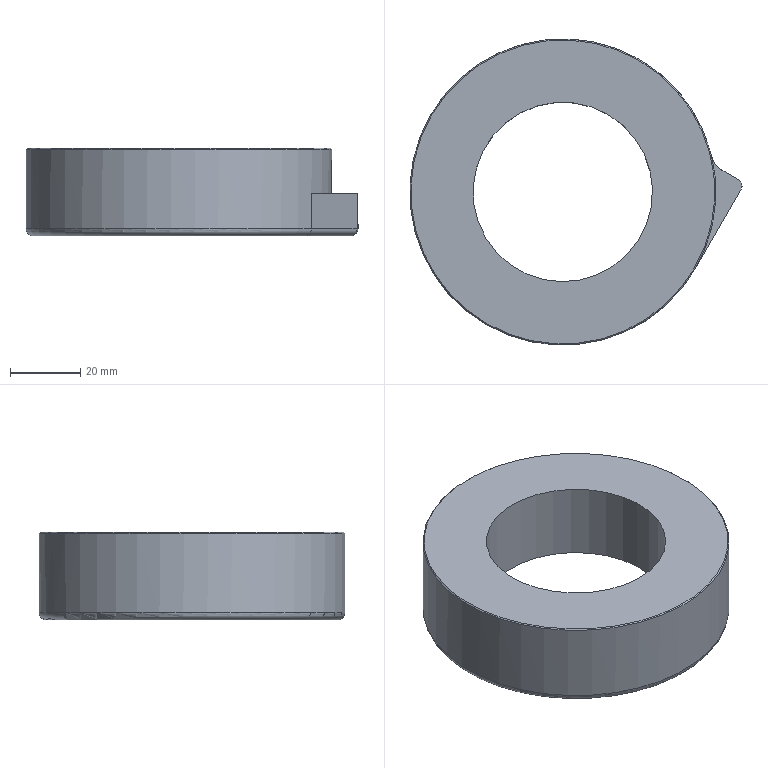Part | STEP file | 1 solid | 26 faces | box 94.44 x 87 x 25 mm | volume 90953 mm3 | plane 9 | cylinder 8 | cone 5 | torus 3 | sphere 1 | commonest cylinder face diameters 4 x3 14 x1 51 x1 71 x1 78.023 x1 87 x1
STEP:
#1=CARTESIAN_POINT('',(-37.672,21.75,-13.25));
#2=VERTEX_POINT('',#1);
#3=CARTESIAN_POINT('',(42.231,10.43,-13.25));
#4=VERTEX_POINT('',#3);
#5=CARTESIAN_POINT('',(0.,0.,-13.25));
#6=DIRECTION('',(0.,0.,-1.));
#7=DIRECTION('',(-0.866,0.5,0.));
#8=AXIS2_PLACEMENT_3D('',#5,#6,#7);
#9=CIRCLE('',#8,43.5);
#10=EDGE_CURVE('',#2,#4,#9,.T.);
#11=ORIENTED_EDGE('',*,*,#10,.T.);
#12=CARTESIAN_POINT('',(40.289,9.951,-15.25));
#13=VERTEX_POINT('',#12);
#14=CARTESIAN_POINT('',(40.289,9.951,-13.25));
#15=DIRECTION('',(-0.2398,0.9708,0.));
#16=DIRECTION('',(0.9708,0.2398,0.));
#17=AXIS2_PLACEMENT_3D('',#14,#15,#16);
#18=CIRCLE('',#17,2.);
#19=EDGE_CURVE('',#4,#13,#18,.T.);
#20=ORIENTED_EDGE('',*,*,#19,.T.);
#21=CARTESIAN_POINT('',(35.94,-20.75,-15.25));
#22=VERTEX_POINT('',#21);
#23=CARTESIAN_POINT('',(0.,0.,-15.25));
#24=DIRECTION('',(0.,0.,-1.));
#25=DIRECTION('',(0.866,-0.5,0.));
#26=AXIS2_PLACEMENT_3D('',#23,#24,#25);
#27=CIRCLE('',#26,41.5);
#28=EDGE_CURVE('',#22,#13,#27,.T.);
#29=ORIENTED_EDGE('',*,*,#28,.F.);
#30=CARTESIAN_POINT('',(37.672,-21.75,-13.25));
#31=VERTEX_POINT('',#30);
#32=CARTESIAN_POINT('',(35.94,-20.75,-13.25));
#33=DIRECTION('',(-0.5,-0.866,0.));
#34=DIRECTION('',(0.,0.,-1.));
#35=AXIS2_PLACEMENT_3D('',#32,#33,#34);
#36=CIRCLE('',#35,2.);
#37=EDGE_CURVE('',#22,#31,#36,.T.);
#38=ORIENTED_EDGE('',*,*,#37,.T.);
#39=CARTESIAN_POINT('',(37.672,-21.75,-13.25));
#40=CARTESIAN_POINT('',(37.217,-22.539,-13.25));
#41=CARTESIAN_POINT('',(36.256,-24.089,-13.25));
#42=CARTESIAN_POINT('',(34.671,-26.318,-13.25));
#43=CARTESIAN_POINT('',(32.95,-28.443,-13.25));
#44=CARTESIAN_POINT('',(31.099,-30.457,-13.25));
#45=CARTESIAN_POINT('',(29.125,-32.35,-13.25));
#46=CARTESIAN_POINT('',(27.036,-34.115,-13.25));
#47=CARTESIAN_POINT('',(24.84,-35.745,-13.25));
#48=CARTESIAN_POINT('',(22.546,-37.235,-13.25));
#49=CARTESIAN_POINT('',(20.163,-38.577,-13.25));
#50=CARTESIAN_POINT('',(17.701,-39.767,-13.25));
#51=CARTESIAN_POINT('',(15.168,-40.8,-13.25));
#52=CARTESIAN_POINT('',(12.576,-41.672,-13.25));
#53=CARTESIAN_POINT('',(9.934,-42.38,-13.25));
#54=CARTESIAN_POINT('',(7.253,-42.92,-13.25));
#55=CARTESIAN_POINT('',(4.543,-43.291,-13.25));
#56=CARTESIAN_POINT('',(1.816,-43.491,-13.25));
#57=CARTESIAN_POINT('',(-0.919,-43.519,-13.25));
#58=CARTESIAN_POINT('',(-3.65,-43.375,-13.25));
#59=CARTESIAN_POINT('',(-6.367,-43.06,-13.25));
#60=CARTESIAN_POINT('',(-9.059,-42.576,-13.25));
#61=CARTESIAN_POINT('',(-11.715,-41.923,-13.25));
#62=CARTESIAN_POINT('',(-14.324,-41.104,-13.25));
#63=CARTESIAN_POINT('',(-16.877,-40.124,-13.25));
#64=CARTESIAN_POINT('',(-19.364,-38.984,-13.25));
#65=CARTESIAN_POINT('',(-21.774,-37.691,-13.25));
#66=CARTESIAN_POINT('',(-24.098,-36.25,-13.25));
#67=CARTESIAN_POINT('',(-26.327,-34.665,-13.25));
#68=CARTESIAN_POINT('',(-28.452,-32.943,-13.25));
#69=CARTESIAN_POINT('',(-30.464,-31.091,-13.25));
#70=CARTESIAN_POINT('',(-32.357,-29.117,-13.25));
#71=CARTESIAN_POINT('',(-34.121,-27.027,-13.25));
#72=CARTESIAN_POINT('',(-35.751,-24.831,-13.25));
#73=CARTESIAN_POINT('',(-37.24,-22.537,-13.25));
#74=CARTESIAN_POINT('',(-38.582,-20.154,-13.25));
#75=CARTESIAN_POINT('',(-39.772,-17.691,-13.25));
#76=CARTESIAN_POINT('',(-40.804,-15.158,-13.25));
#77=CARTESIAN_POINT('',(-41.675,-12.566,-13.25));
#78=CARTESIAN_POINT('',(-42.382,-9.924,-13.25));
#79=CARTESIAN_POINT('',(-42.922,-7.242,-13.25));
#80=CARTESIAN_POINT('',(-43.292,-4.533,-13.25));
#81=CARTESIAN_POINT('',(-43.491,-1.805,-13.25));
#82=CARTESIAN_POINT('',(-43.519,0.9299,-13.25));
#83=CARTESIAN_POINT('',(-43.374,3.661,-13.25));
#84=CARTESIAN_POINT('',(-43.059,6.378,-13.25));
#85=CARTESIAN_POINT('',(-42.573,9.069,-13.25));
#86=CARTESIAN_POINT('',(-41.92,11.725,-13.25));
#87=CARTESIAN_POINT('',(-41.101,14.334,-13.25));
#88=CARTESIAN_POINT('',(-40.119,16.887,-13.25));
#89=CARTESIAN_POINT('',(-39.013,19.301,-13.25));
#90=CARTESIAN_POINT('',(-38.193,20.839,-13.25));
#91=CARTESIAN_POINT('',(-37.781,21.561,-13.25));
#92=CARTESIAN_POINT('',(-37.745,21.624,-13.25));
#93=CARTESIAN_POINT('',(-37.708,21.687,-13.25));
#94=CARTESIAN_POINT('',(-37.672,21.75,-13.25));
#95=B_SPLINE_CURVE_WITH_KNOTS('',3,(#39,#40,#41,#42,#43,#44,#45,#46,#47,#48,#49,#50,#51,#52,#53,#54,#55,#56,#57,#58,#59,#60,#61,#62,#63,#64,#65,#66,#67,#68,#69,#70,#71,#72,#73,#74,#75,#76,#77,#78,#79,#80,#81,#82,#83,#84,#85,#86,#87,#88,#89,#90,#91,#92,#93,#94),.UNSPECIFIED.,.F.,.F.,(4,1,1,1,1,1,1,1,1,1,1,1,1,1,1,1,1,1,1,1,1,1,1,1,1,1,1,1,1,1,1,1,1,1,1,1,1,1,1,1,1,1,1,1,1,1,1,1,1,1,3,4),(0.,0.02,0.04001,0.06001,0.08001,0.1,0.12,0.14,0.16,0.18,0.2,0.22,0.24,0.26,0.28,0.3,0.3201,0.3401,0.3601,0.3801,0.4001,0.4201,0.4401,0.4601,0.4801,0.5001,0.5201,0.5401,0.5601,0.5801,0.6001,0.6201,0.6401,0.6601,0.6801,0.7001,0.7201,0.7401,0.7601,0.7801,0.8001,0.8201,0.8401,0.8601,0.8801,0.9001,0.9201,0.9401,0.9602,0.9802,0.9984,1.),.UNSPECIFIED.);
#96=EDGE_CURVE('',#31,#2,#95,.T.);
#97=ORIENTED_EDGE('',*,*,#96,.T.);
#98=EDGE_LOOP('',(#11,#20,#29,#38,#97));
#99=FACE_BOUND('',#98,.T.);
#100=CARTESIAN_POINT('',(0.,0.,-13.25));
#101=DIRECTION('',(0.,0.,1.));
#102=DIRECTION('',(-0.8685,0.4956,0.));
#103=AXIS2_PLACEMENT_3D('',#100,#101,#102);
#104=TOROIDAL_SURFACE('',#103,41.5,2.);
#105=ADVANCED_FACE('',(#99),#104,.T.);
#106=ORIENTED_EDGE('',*,*,#28,.T.);
#107=CARTESIAN_POINT('',(44.527,4.315,-15.25));
#108=VERTEX_POINT('',#107);
#109=CARTESIAN_POINT('',(49.027,12.109,-15.25));
#110=DIRECTION('',(0.,0.,1.));
#111=DIRECTION('',(-0.9708,-0.2398,0.));
#112=AXIS2_PLACEMENT_3D('',#109,#110,#111);
#113=CIRCLE('',#112,9.);
#114=EDGE_CURVE('',#13,#108,#113,.T.);
#115=ORIENTED_EDGE('',*,*,#114,.T.);
#116=CARTESIAN_POINT('',(48.94,1.767,-15.25));
#117=VERTEX_POINT('',#116);
#118=CARTESIAN_POINT('',(48.94,1.767,-15.25));
#119=DIRECTION('',(-0.866,0.5,0.));
#120=VECTOR('',#119,1.);
#121=LINE('',#118,#120);
#122=EDGE_CURVE('',#117,#108,#121,.T.);
#123=ORIENTED_EDGE('',*,*,#122,.F.);
#124=CARTESIAN_POINT('',(35.94,-20.75,-15.25));
#125=DIRECTION('',(0.5,0.866,0.));
#126=VECTOR('',#125,1.);
#127=LINE('',#124,#126);
#128=EDGE_CURVE('',#22,#117,#127,.T.);
#129=ORIENTED_EDGE('',*,*,#128,.F.);
#130=EDGE_LOOP('',(#106,#115,#123,#129));
#131=FACE_BOUND('',#130,.T.);
#132=CARTESIAN_POINT('',(31.004,-17.9,-15.25));
#133=VERTEX_POINT('',#132);
#134=CARTESIAN_POINT('',(0.,0.,-15.25));
#135=DIRECTION('',(0.,0.,1.));
#136=DIRECTION('',(1.,0.,0.));
#137=AXIS2_PLACEMENT_3D('',#134,#135,#136);
#138=CIRCLE('',#137,35.8);
#139=EDGE_CURVE('',#133,#133,#138,.T.);
#140=ORIENTED_EDGE('',*,*,#139,.T.);
#141=EDGE_LOOP('',(#140));
#142=FACE_BOUND('',#141,.T.);
#143=CARTESIAN_POINT('',(-35.724,-20.625,-15.25));
#144=VERTEX_POINT('',#143);
#145=CARTESIAN_POINT('',(-34.425,-19.875,-15.25));
#146=VERTEX_POINT('',#145);
#147=CARTESIAN_POINT('',(-35.074,-20.25,-15.25));
#148=DIRECTION('',(0.,0.,1.));
#149=DIRECTION('',(-0.866,-0.5,0.));
#150=AXIS2_PLACEMENT_3D('',#147,#148,#149);
#151=CIRCLE('',#150,0.75);
#152=EDGE_CURVE('',#144,#146,#151,.T.);
#153=ORIENTED_EDGE('',*,*,#152,.T.);
#154=CARTESIAN_POINT('',(-35.074,-20.25,-15.25));
#155=DIRECTION('',(0.,0.,1.));
#156=DIRECTION('',(0.866,0.5,0.));
#157=AXIS2_PLACEMENT_3D('',#154,#155,#156);
#158=CIRCLE('',#157,0.75);
#159=EDGE_CURVE('',#146,#144,#158,.T.);
#160=ORIENTED_EDGE('',*,*,#159,.T.);
#161=EDGE_LOOP('',(#153,#160));
#162=FACE_BOUND('',#161,.T.);
#163=CARTESIAN_POINT('',(0.,0.,-15.25));
#164=DIRECTION('',(0.,0.,1.));
#165=DIRECTION('',(1.,0.,0.));
#166=AXIS2_PLACEMENT_3D('',#163,#164,#165);
#167=PLANE('',#166);
#168=ADVANCED_FACE('',(#131,#142,#162),#167,.F.);
#169=CARTESIAN_POINT('',(50.672,0.7667,-13.25));
#170=VERTEX_POINT('',#169);
#171=CARTESIAN_POINT('',(50.672,0.7667,-13.25));
#172=DIRECTION('',(-0.5,-0.866,0.));
#173=VECTOR('',#172,1.);
#174=LINE('',#171,#173);
#175=EDGE_CURVE('',#170,#31,#174,.T.);
#176=ORIENTED_EDGE('',*,*,#175,.T.);
#177=ORIENTED_EDGE('',*,*,#37,.F.);
#178=ORIENTED_EDGE('',*,*,#128,.T.);
#179=CARTESIAN_POINT('',(48.94,1.767,-13.25));
#180=DIRECTION('',(0.5,0.866,0.));
#181=DIRECTION('',(0.866,-0.5,0.));
#182=AXIS2_PLACEMENT_3D('',#179,#180,#181);
#183=CIRCLE('',#182,2.);
#184=EDGE_CURVE('',#170,#117,#183,.T.);
#185=ORIENTED_EDGE('',*,*,#184,.F.);
#186=EDGE_LOOP('',(#176,#177,#178,#185));
#187=FACE_BOUND('',#186,.T.);
#188=CARTESIAN_POINT('',(57.805,17.121,-13.25));
#189=DIRECTION('',(0.5,0.866,0.));
#190=DIRECTION('',(0.,0.,-1.));
#191=AXIS2_PLACEMENT_3D('',#188,#189,#190);
#192=CYLINDRICAL_SURFACE('',#191,2.);
#193=ADVANCED_FACE('',(#187),#192,.T.);
#194=ORIENTED_EDGE('',*,*,#184,.T.);
#195=CARTESIAN_POINT('',(49.94,3.499,-13.25));
#196=VERTEX_POINT('',#195);
#197=CARTESIAN_POINT('',(48.94,1.767,-13.25));
#198=DIRECTION('',(0.866,-0.5,0.));
#199=DIRECTION('',(0.,0.,-1.));
#200=AXIS2_PLACEMENT_3D('',#197,#198,#199);
#201=CIRCLE('',#200,2.);
#202=EDGE_CURVE('',#117,#196,#201,.T.);
#203=ORIENTED_EDGE('',*,*,#202,.T.);
#204=CARTESIAN_POINT('',(48.94,1.767,-13.25));
#205=DIRECTION('',(0.,0.,-1.));
#206=DIRECTION('',(0.5,0.866,0.));
#207=AXIS2_PLACEMENT_3D('',#204,#205,#206);
#208=CIRCLE('',#207,2.);
#209=EDGE_CURVE('',#196,#170,#208,.T.);
#210=ORIENTED_EDGE('',*,*,#209,.T.);
#211=EDGE_LOOP('',(#194,#203,#210));
#212=FACE_BOUND('',#211,.T.);
#213=CARTESIAN_POINT('',(48.94,1.767,-13.25));
#214=DIRECTION('',(0.5,0.866,0.));
#215=DIRECTION('',(0.,0.,1.));
#216=AXIS2_PLACEMENT_3D('',#213,#214,#215);
#217=SPHERICAL_SURFACE('',#216,2.);
#218=ADVANCED_FACE('',(#212),#217,.T.);
#219=CARTESIAN_POINT('',(50.491,3.03,-8.25));
#220=VERTEX_POINT('',#219);
#221=CARTESIAN_POINT('',(49.94,3.499,-10.321));
#222=VERTEX_POINT('',#221);
#223=CARTESIAN_POINT('',(50.491,3.03,-8.25));
#224=CARTESIAN_POINT('',(50.491,3.03,-8.283));
#225=CARTESIAN_POINT('',(50.49,3.03,-8.349));
#226=CARTESIAN_POINT('',(50.487,3.034,-8.447));
#227=CARTESIAN_POINT('',(50.483,3.039,-8.543));
#228=CARTESIAN_POINT('',(50.476,3.047,-8.639));
#229=CARTESIAN_POINT('',(50.468,3.057,-8.733));
#230=CARTESIAN_POINT('',(50.459,3.068,-8.825));
#231=CARTESIAN_POINT('',(50.448,3.081,-8.916));
#232=CARTESIAN_POINT('',(50.435,3.096,-9.005));
#233=CARTESIAN_POINT('',(50.42,3.112,-9.093));
#234=CARTESIAN_POINT('',(50.404,3.129,-9.179));
#235=CARTESIAN_POINT('',(50.387,3.148,-9.262));
#236=CARTESIAN_POINT('',(50.368,3.167,-9.343));
#237=CARTESIAN_POINT('',(50.348,3.187,-9.421));
#238=CARTESIAN_POINT('',(50.328,3.207,-9.496));
#239=CARTESIAN_POINT('',(50.306,3.228,-9.567));
#240=CARTESIAN_POINT('',(50.284,3.248,-9.636));
#241=CARTESIAN_POINT('',(50.261,3.269,-9.701));
#242=CARTESIAN_POINT('',(50.237,3.289,-9.763));
#243=CARTESIAN_POINT('',(50.214,3.308,-9.821));
#244=CARTESIAN_POINT('',(50.191,3.327,-9.876));
#245=CARTESIAN_POINT('',(50.168,3.345,-9.926));
#246=CARTESIAN_POINT('',(50.146,3.362,-9.974));
#247=CARTESIAN_POINT('',(50.124,3.379,-10.018));
#248=CARTESIAN_POINT('',(50.102,3.394,-10.059));
#249=CARTESIAN_POINT('',(50.081,3.409,-10.098));
#250=CARTESIAN_POINT('',(50.06,3.424,-10.135));
#251=CARTESIAN_POINT('',(50.04,3.437,-10.17));
#252=CARTESIAN_POINT('',(50.02,3.45,-10.203));
#253=CARTESIAN_POINT('',(50.,3.463,-10.234));
#254=CARTESIAN_POINT('',(49.98,3.475,-10.264));
#255=CARTESIAN_POINT('',(49.96,3.487,-10.293));
#256=CARTESIAN_POINT('',(49.947,3.495,-10.312));
#257=CARTESIAN_POINT('',(49.94,3.499,-10.321));
#258=B_SPLINE_CURVE_WITH_KNOTS('',3,(#223,#224,#225,#226,#227,#228,#229,#230,#231,#232,#233,#234,#235,#236,#237,#238,#239,#240,#241,#242,#243,#244,#245,#246,#247,#248,#249,#250,#251,#252,#253,#254,#255,#256,#257),.UNSPECIFIED.,.F.,.F.,(4,1,1,1,1,1,1,1,1,1,1,1,1,1,1,1,1,1,1,1,1,1,1,1,1,1,1,1,1,1,1,1,4),(0.,0.04051,0.08112,0.1217,0.162,0.202,0.2417,0.2813,0.3207,0.36,0.399,0.4375,0.4751,0.5122,0.5481,0.5832,0.6171,0.6505,0.6824,0.713,0.7417,0.7696,0.7954,0.82,0.8429,0.8655,0.8868,0.9074,0.9269,0.946,0.9644,0.9824,1.),.UNSPECIFIED.);
#259=EDGE_CURVE('',#220,#222,#258,.T.);
#260=ORIENTED_EDGE('',*,*,#259,.F.);
#261=CARTESIAN_POINT('',(49.94,3.499,-6.179));
#262=VERTEX_POINT('',#261);
#263=CARTESIAN_POINT('',(49.94,3.499,-6.179));
#264=CARTESIAN_POINT('',(49.954,3.491,-6.198));
#265=CARTESIAN_POINT('',(49.98,3.475,-6.236));
#266=CARTESIAN_POINT('',(50.018,3.451,-6.295));
#267=CARTESIAN_POINT('',(50.054,3.428,-6.355));
#268=CARTESIAN_POINT('',(50.089,3.404,-6.416));
#269=CARTESIAN_POINT('',(50.122,3.38,-6.478));
#270=CARTESIAN_POINT('',(50.154,3.357,-6.542));
#271=CARTESIAN_POINT('',(50.184,3.333,-6.607));
#272=CARTESIAN_POINT('',(50.212,3.31,-6.674));
#273=CARTESIAN_POINT('',(50.24,3.287,-6.742));
#274=CARTESIAN_POINT('',(50.265,3.265,-6.812));
#275=CARTESIAN_POINT('',(50.29,3.243,-6.882));
#276=CARTESIAN_POINT('',(50.312,3.222,-6.953));
#277=CARTESIAN_POINT('',(50.333,3.202,-7.024));
#278=CARTESIAN_POINT('',(50.353,3.183,-7.096));
#279=CARTESIAN_POINT('',(50.371,3.164,-7.168));
#280=CARTESIAN_POINT('',(50.387,3.147,-7.239));
#281=CARTESIAN_POINT('',(50.402,3.132,-7.31));
#282=CARTESIAN_POINT('',(50.415,3.117,-7.381));
#283=CARTESIAN_POINT('',(50.427,3.104,-7.451));
#284=CARTESIAN_POINT('',(50.438,3.092,-7.519));
#285=CARTESIAN_POINT('',(50.448,3.081,-7.585));
#286=CARTESIAN_POINT('',(50.456,3.071,-7.651));
#287=CARTESIAN_POINT('',(50.463,3.063,-7.714));
#288=CARTESIAN_POINT('',(50.469,3.056,-7.777));
#289=CARTESIAN_POINT('',(50.475,3.049,-7.838));
#290=CARTESIAN_POINT('',(50.479,3.044,-7.899));
#291=CARTESIAN_POINT('',(50.483,3.039,-7.959));
#292=CARTESIAN_POINT('',(50.486,3.036,-8.018));
#293=CARTESIAN_POINT('',(50.488,3.033,-8.077));
#294=CARTESIAN_POINT('',(50.49,3.031,-8.135));
#295=CARTESIAN_POINT('',(50.491,3.03,-8.193));
#296=CARTESIAN_POINT('',(50.491,3.03,-8.231));
#297=CARTESIAN_POINT('',(50.491,3.03,-8.25));
#298=B_SPLINE_CURVE_WITH_KNOTS('',3,(#263,#264,#265,#266,#267,#268,#269,#270,#271,#272,#273,#274,#275,#276,#277,#278,#279,#280,#281,#282,#283,#284,#285,#286,#287,#288,#289,#290,#291,#292,#293,#294,#295,#296,#297),.UNSPECIFIED.,.F.,.F.,(4,1,1,1,1,1,1,1,1,1,1,1,1,1,1,1,1,1,1,1,1,1,1,1,1,1,1,1,1,1,1,1,4),(0.,0.03654,0.07276,0.1087,0.1445,0.1802,0.2158,0.2514,0.2871,0.3229,0.3585,0.3941,0.4292,0.4641,0.4984,0.5324,0.5656,0.5986,0.6306,0.6619,0.692,0.7216,0.7498,0.7774,0.8039,0.8301,0.8557,0.8808,0.9052,0.9295,0.9533,0.9768,1.),.UNSPECIFIED.);
#299=EDGE_CURVE('',#262,#220,#298,.T.);
#300=ORIENTED_EDGE('',*,*,#299,.F.);
#301=CARTESIAN_POINT('',(49.94,3.499,-3.25));
#302=VERTEX_POINT('',#301);
#303=CARTESIAN_POINT('',(49.94,3.499,-6.179));
#304=DIRECTION('',(0.,0.,1.));
#305=VECTOR('',#304,1.);
#306=LINE('',#303,#305);
#307=EDGE_CURVE('',#262,#302,#306,.T.);
#308=ORIENTED_EDGE('',*,*,#307,.T.);
#309=CARTESIAN_POINT('',(50.672,0.7667,-3.25));
#310=VERTEX_POINT('',#309);
#311=CARTESIAN_POINT('',(48.94,1.767,-3.25));
#312=DIRECTION('',(0.,0.,1.));
#313=DIRECTION('',(0.866,-0.5,0.));
#314=AXIS2_PLACEMENT_3D('',#311,#312,#313);
#315=CIRCLE('',#314,2.);
#316=EDGE_CURVE('',#310,#302,#315,.T.);
#317=ORIENTED_EDGE('',*,*,#316,.F.);
#318=CARTESIAN_POINT('',(50.672,0.7667,-3.25));
#319=DIRECTION('',(0.,0.,-1.));
#320=VECTOR('',#319,1.);
#321=LINE('',#318,#320);
#322=EDGE_CURVE('',#310,#170,#321,.T.);
#323=ORIENTED_EDGE('',*,*,#322,.T.);
#324=ORIENTED_EDGE('',*,*,#209,.F.);
#325=CARTESIAN_POINT('',(49.94,3.499,-13.25));
#326=DIRECTION('',(0.,0.,1.));
#327=VECTOR('',#326,1.);
#328=LINE('',#325,#327);
#329=EDGE_CURVE('',#196,#222,#328,.T.);
#330=ORIENTED_EDGE('',*,*,#329,.T.);
#331=EDGE_LOOP('',(#260,#300,#308,#317,#323,#324,#330));
#332=FACE_BOUND('',#331,.T.);
#333=CARTESIAN_POINT('',(48.94,1.767,-15.25));
#334=DIRECTION('',(0.,0.,1.));
#335=DIRECTION('',(0.5,0.866,0.));
#336=AXIS2_PLACEMENT_3D('',#333,#334,#335);
#337=CYLINDRICAL_SURFACE('',#336,2.);
#338=ADVANCED_FACE('',(#332),#337,.T.);
#339=CARTESIAN_POINT('',(45.527,6.047,-10.199));
#340=VERTEX_POINT('',#339);
#341=CARTESIAN_POINT('',(47.775,4.749,-8.25));
#342=DIRECTION('',(-0.5,-0.866,0.));
#343=DIRECTION('',(-0.6925,0.3998,-0.6005));
#344=AXIS2_PLACEMENT_3D('',#341,#342,#343);
#345=CIRCLE('',#344,3.246);
#346=EDGE_CURVE('',#340,#222,#345,.T.);
#347=ORIENTED_EDGE('',*,*,#346,.T.);
#348=ORIENTED_EDGE('',*,*,#329,.F.);
#349=CARTESIAN_POINT('',(45.527,6.047,-13.25));
#350=VERTEX_POINT('',#349);
#351=CARTESIAN_POINT('',(45.527,6.047,-13.25));
#352=DIRECTION('',(0.866,-0.5,0.));
#353=VECTOR('',#352,1.);
#354=LINE('',#351,#353);
#355=EDGE_CURVE('',#350,#196,#354,.T.);
#356=ORIENTED_EDGE('',*,*,#355,.F.);
#357=CARTESIAN_POINT('',(45.527,6.047,-10.199));
#358=DIRECTION('',(0.,0.,-1.));
#359=VECTOR('',#358,1.);
#360=LINE('',#357,#359);
#361=EDGE_CURVE('',#340,#350,#360,.T.);
#362=ORIENTED_EDGE('',*,*,#361,.F.);
#363=EDGE_LOOP('',(#347,#348,#356,#362));
#364=FACE_BOUND('',#363,.T.);
#365=CARTESIAN_POINT('',(49.94,3.499,-15.25));
#366=DIRECTION('',(-0.5,-0.866,0.));
#367=DIRECTION('',(-0.866,0.5,0.));
#368=AXIS2_PLACEMENT_3D('',#365,#366,#367);
#369=PLANE('',#368);
#370=ADVANCED_FACE('',(#364),#369,.F.);
#371=CARTESIAN_POINT('',(45.527,6.047,-3.25));
#372=VERTEX_POINT('',#371);
#373=CARTESIAN_POINT('',(42.231,10.43,-3.25));
#374=VERTEX_POINT('',#373);
#375=CARTESIAN_POINT('',(49.027,12.109,-3.25));
#376=DIRECTION('',(0.,0.,-1.));
#377=DIRECTION('',(-0.5,-0.866,0.));
#378=AXIS2_PLACEMENT_3D('',#375,#376,#377);
#379=CIRCLE('',#378,7.);
#380=EDGE_CURVE('',#372,#374,#379,.T.);
#381=ORIENTED_EDGE('',*,*,#380,.F.);
#382=CARTESIAN_POINT('',(45.527,6.047,-6.301));
#383=VERTEX_POINT('',#382);
#384=CARTESIAN_POINT('',(45.527,6.047,-3.25));
#385=DIRECTION('',(0.,0.,-1.));
#386=VECTOR('',#385,1.);
#387=LINE('',#384,#386);
#388=EDGE_CURVE('',#372,#383,#387,.T.);
#389=ORIENTED_EDGE('',*,*,#388,.T.);
#390=CARTESIAN_POINT('',(45.527,6.047,-6.301));
#391=CARTESIAN_POINT('',(45.51,6.056,-6.326));
#392=CARTESIAN_POINT('',(45.478,6.075,-6.376));
#393=CARTESIAN_POINT('',(45.433,6.102,-6.454));
#394=CARTESIAN_POINT('',(45.39,6.128,-6.531));
#395=CARTESIAN_POINT('',(45.349,6.153,-6.61));
#396=CARTESIAN_POINT('',(45.306,6.18,-6.698));
#397=CARTESIAN_POINT('',(45.262,6.207,-6.797));
#398=CARTESIAN_POINT('',(45.218,6.236,-6.905));
#399=CARTESIAN_POINT('',(45.181,6.26,-7.005));
#400=CARTESIAN_POINT('',(45.15,6.28,-7.096));
#401=CARTESIAN_POINT('',(45.125,6.297,-7.178));
#402=CARTESIAN_POINT('',(45.102,6.313,-7.259));
#403=CARTESIAN_POINT('',(45.08,6.328,-7.343));
#404=CARTESIAN_POINT('',(45.059,6.342,-7.432));
#405=CARTESIAN_POINT('',(45.037,6.357,-7.541));
#406=CARTESIAN_POINT('',(45.015,6.372,-7.668));
#407=CARTESIAN_POINT('',(44.996,6.386,-7.808));
#408=CARTESIAN_POINT('',(44.984,6.394,-7.934));
#409=CARTESIAN_POINT('',(44.977,6.399,-8.042));
#410=CARTESIAN_POINT('',(44.973,6.402,-8.129));
#411=CARTESIAN_POINT('',(44.972,6.403,-8.197));
#412=CARTESIAN_POINT('',(44.972,6.403,-8.249));
#413=CARTESIAN_POINT('',(44.972,6.403,-8.309));
#414=CARTESIAN_POINT('',(44.974,6.402,-8.391));
#415=CARTESIAN_POINT('',(44.979,6.398,-8.495));
#416=CARTESIAN_POINT('',(44.987,6.392,-8.598));
#417=CARTESIAN_POINT('',(44.999,6.384,-8.71));
#418=CARTESIAN_POINT('',(45.015,6.372,-8.832));
#419=CARTESIAN_POINT('',(45.037,6.357,-8.958));
#420=CARTESIAN_POINT('',(45.064,6.339,-9.088));
#421=CARTESIAN_POINT('',(45.099,6.315,-9.234));
#422=CARTESIAN_POINT('',(45.149,6.281,-9.406));
#423=CARTESIAN_POINT('',(45.209,6.241,-9.575));
#424=CARTESIAN_POINT('',(45.265,6.205,-9.712));
#425=CARTESIAN_POINT('',(45.305,6.18,-9.8));
#426=CARTESIAN_POINT('',(45.334,6.162,-9.859));
#427=CARTESIAN_POINT('',(45.357,6.148,-9.906));
#428=CARTESIAN_POINT('',(45.381,6.133,-9.952));
#429=CARTESIAN_POINT('',(45.408,6.117,-10.001));
#430=CARTESIAN_POINT('',(45.437,6.099,-10.053));
#431=CARTESIAN_POINT('',(45.469,6.08,-10.108));
#432=CARTESIAN_POINT('',(45.499,6.063,-10.156));
#433=CARTESIAN_POINT('',(45.518,6.052,-10.187));
#434=CARTESIAN_POINT('',(45.527,6.047,-10.199));
#435=B_SPLINE_CURVE_WITH_KNOTS('',3,(#390,#391,#392,#393,#394,#395,#396,#397,#398,#399,#400,#401,#402,#403,#404,#405,#406,#407,#408,#409,#410,#411,#412,#413,#414,#415,#416,#417,#418,#419,#420,#421,#422,#423,#424,#425,#426,#427,#428,#429,#430,#431,#432,#433,#434),.UNSPECIFIED.,.F.,.F.,(4,1,1,1,1,1,1,1,1,1,1,1,1,1,1,1,1,1,1,1,1,1,1,1,1,1,1,1,1,1,1,1,1,1,1,1,1,1,1,1,1,1,4),(0.,0.02258,0.04492,0.06707,0.08901,0.1109,0.1399,0.1686,0.1971,0.2181,0.239,0.2595,0.2798,0.3019,0.326,0.3603,0.3943,0.4281,0.451,0.4717,0.4903,0.5,0.5089,0.5336,0.5585,0.5833,0.6081,0.6391,0.6719,0.7003,0.7353,0.7805,0.831,0.8669,0.8892,0.9026,0.9158,0.9286,0.9411,0.9572,0.973,0.9886,1.),.UNSPECIFIED.);
#436=EDGE_CURVE('',#383,#340,#435,.T.);
#437=ORIENTED_EDGE('',*,*,#436,.T.);
#438=ORIENTED_EDGE('',*,*,#361,.T.);
#439=CARTESIAN_POINT('',(49.027,12.109,-13.25));
#440=DIRECTION('',(0.,0.,1.));
#441=DIRECTION('',(-0.9708,-0.2398,0.));
#442=AXIS2_PLACEMENT_3D('',#439,#440,#441);
#443=CIRCLE('',#442,7.);
#444=EDGE_CURVE('',#4,#350,#443,.T.);
#445=ORIENTED_EDGE('',*,*,#444,.F.);
#446=CARTESIAN_POINT('',(42.231,10.43,-3.25));
#447=DIRECTION('',(0.,0.,-1.));
#448=VECTOR('',#447,1.);
#449=LINE('',#446,#448);
#450=EDGE_CURVE('',#374,#4,#449,.T.);
#451=ORIENTED_EDGE('',*,*,#450,.F.);
#452=EDGE_LOOP('',(#381,#389,#437,#438,#445,#451));
#453=FACE_BOUND('',#452,.T.);
#454=CARTESIAN_POINT('',(49.027,12.109,-15.25));
#455=DIRECTION('',(0.,0.,1.));
#456=DIRECTION('',(0.5,0.866,0.));
#457=AXIS2_PLACEMENT_3D('',#454,#455,#456);
#458=CYLINDRICAL_SURFACE('',#457,7.);
#459=ADVANCED_FACE('',(#453),#458,.F.);
#460=ORIENTED_EDGE('',*,*,#450,.T.);
#461=ORIENTED_EDGE('',*,*,#10,.F.);
#462=ORIENTED_EDGE('',*,*,#96,.F.);
#463=CARTESIAN_POINT('',(37.672,-21.75,-3.25));
#464=VERTEX_POINT('',#463);
#465=CARTESIAN_POINT('',(37.672,-21.75,-13.25));
#466=DIRECTION('',(0.,0.,1.));
#467=VECTOR('',#466,1.);
#468=LINE('',#465,#467);
#469=EDGE_CURVE('',#31,#464,#468,.T.);
#470=ORIENTED_EDGE('',*,*,#469,.T.);
#471=CARTESIAN_POINT('',(0.,0.,-3.25));
#472=DIRECTION('',(0.,0.,-1.));
#473=DIRECTION('',(0.9708,0.2398,0.));
#474=AXIS2_PLACEMENT_3D('',#471,#472,#473);
#475=CIRCLE('',#474,43.5);
#476=EDGE_CURVE('',#374,#464,#475,.T.);
#477=ORIENTED_EDGE('',*,*,#476,.F.);
#478=EDGE_LOOP('',(#460,#461,#462,#470,#477));
#479=FACE_BOUND('',#478,.T.);
#480=CARTESIAN_POINT('',(-37.672,21.75,9.45));
#481=VERTEX_POINT('',#480);
#482=CARTESIAN_POINT('',(-37.672,21.75,9.45));
#483=CARTESIAN_POINT('',(-38.128,20.961,9.45));
#484=CARTESIAN_POINT('',(-38.989,19.354,9.45));
#485=CARTESIAN_POINT('',(-40.128,16.867,9.45));
#486=CARTESIAN_POINT('',(-41.108,14.314,9.45));
#487=CARTESIAN_POINT('',(-41.926,11.704,9.45));
#488=CARTESIAN_POINT('',(-42.578,9.048,9.45));
#489=CARTESIAN_POINT('',(-43.062,6.356,9.45));
#490=CARTESIAN_POINT('',(-43.376,3.639,9.45));
#491=CARTESIAN_POINT('',(-43.519,0.9081,9.45));
#492=CARTESIAN_POINT('',(-43.49,-1.827,9.45));
#493=CARTESIAN_POINT('',(-43.29,-4.554,9.45));
#494=CARTESIAN_POINT('',(-42.918,-7.264,9.45));
#495=CARTESIAN_POINT('',(-42.377,-9.945,9.45));
#496=CARTESIAN_POINT('',(-41.669,-12.587,9.45));
#497=CARTESIAN_POINT('',(-40.796,-15.179,9.45));
#498=CARTESIAN_POINT('',(-39.763,-17.711,9.45));
#499=CARTESIAN_POINT('',(-38.572,-20.173,9.45));
#500=CARTESIAN_POINT('',(-37.229,-22.555,9.45));
#501=CARTESIAN_POINT('',(-35.739,-24.849,9.45));
#502=CARTESIAN_POINT('',(-34.108,-27.044,9.45));
#503=CARTESIAN_POINT('',(-32.342,-29.133,9.45));
#504=CARTESIAN_POINT('',(-30.449,-31.106,9.45));
#505=CARTESIAN_POINT('',(-28.435,-32.957,9.45));
#506=CARTESIAN_POINT('',(-26.309,-34.678,9.45));
#507=CARTESIAN_POINT('',(-24.08,-36.262,9.45));
#508=CARTESIAN_POINT('',(-21.755,-37.702,9.45));
#509=CARTESIAN_POINT('',(-19.344,-38.994,9.45));
#510=CARTESIAN_POINT('',(-16.857,-40.132,9.45));
#511=CARTESIAN_POINT('',(-14.304,-41.111,9.45));
#512=CARTESIAN_POINT('',(-11.694,-41.929,9.45));
#513=CARTESIAN_POINT('',(-9.037,-42.58,9.45));
#514=CARTESIAN_POINT('',(-6.345,-43.064,9.45));
#515=CARTESIAN_POINT('',(-3.629,-43.377,9.45));
#516=CARTESIAN_POINT('',(-0.8972,-43.519,9.45));
#517=CARTESIAN_POINT('',(1.838,-43.49,9.45));
#518=CARTESIAN_POINT('',(4.565,-43.289,9.45));
#519=CARTESIAN_POINT('',(7.275,-42.916,9.45));
#520=CARTESIAN_POINT('',(9.955,-42.375,9.45));
#521=CARTESIAN_POINT('',(12.597,-41.666,9.45));
#522=CARTESIAN_POINT('',(15.189,-40.793,9.45));
#523=CARTESIAN_POINT('',(17.721,-39.758,9.45));
#524=CARTESIAN_POINT('',(20.182,-38.567,9.45));
#525=CARTESIAN_POINT('',(22.565,-37.223,9.45));
#526=CARTESIAN_POINT('',(24.858,-35.733,9.45));
#527=CARTESIAN_POINT('',(27.053,-34.101,9.45));
#528=CARTESIAN_POINT('',(29.141,-32.335,9.45));
#529=CARTESIAN_POINT('',(31.114,-30.441,9.45));
#530=CARTESIAN_POINT('',(32.964,-28.427,9.45));
#531=CARTESIAN_POINT('',(34.684,-26.301,9.45));
#532=CARTESIAN_POINT('',(36.264,-24.077,9.45));
#533=CARTESIAN_POINT('',(37.22,-22.533,9.45));
#534=CARTESIAN_POINT('',(37.672,-21.75,9.45));
#535=CARTESIAN_POINT('',(38.128,-20.961,9.45));
#536=CARTESIAN_POINT('',(38.989,-19.354,9.45));
#537=CARTESIAN_POINT('',(40.128,-16.867,9.45));
#538=CARTESIAN_POINT('',(41.108,-14.314,9.45));
#539=CARTESIAN_POINT('',(41.926,-11.704,9.45));
#540=CARTESIAN_POINT('',(42.578,-9.048,9.45));
#541=CARTESIAN_POINT('',(43.062,-6.356,9.45));
#542=CARTESIAN_POINT('',(43.376,-3.639,9.45));
#543=CARTESIAN_POINT('',(43.519,-0.9081,9.45));
#544=CARTESIAN_POINT('',(43.49,1.827,9.45));
#545=CARTESIAN_POINT('',(43.29,4.554,9.45));
#546=CARTESIAN_POINT('',(42.918,7.264,9.45));
#547=CARTESIAN_POINT('',(42.377,9.945,9.45));
#548=CARTESIAN_POINT('',(41.669,12.587,9.45));
#549=CARTESIAN_POINT('',(40.796,15.179,9.45));
#550=CARTESIAN_POINT('',(39.763,17.711,9.45));
#551=CARTESIAN_POINT('',(38.572,20.173,9.45));
#552=CARTESIAN_POINT('',(37.229,22.555,9.45));
#553=CARTESIAN_POINT('',(35.739,24.849,9.45));
#554=CARTESIAN_POINT('',(34.108,27.044,9.45));
#555=CARTESIAN_POINT('',(32.342,29.133,9.45));
#556=CARTESIAN_POINT('',(30.449,31.106,9.45));
#557=CARTESIAN_POINT('',(28.435,32.957,9.45));
#558=CARTESIAN_POINT('',(26.309,34.678,9.45));
#559=CARTESIAN_POINT('',(24.08,36.262,9.45));
#560=CARTESIAN_POINT('',(21.755,37.702,9.45));
#561=CARTESIAN_POINT('',(19.344,38.994,9.45));
#562=CARTESIAN_POINT('',(16.857,40.132,9.45));
#563=CARTESIAN_POINT('',(14.304,41.111,9.45));
#564=CARTESIAN_POINT('',(11.694,41.929,9.45));
#565=CARTESIAN_POINT('',(9.037,42.58,9.45));
#566=CARTESIAN_POINT('',(6.345,43.064,9.45));
#567=CARTESIAN_POINT('',(3.629,43.377,9.45));
#568=CARTESIAN_POINT('',(0.8972,43.519,9.45));
#569=CARTESIAN_POINT('',(-1.838,43.49,9.45));
#570=CARTESIAN_POINT('',(-4.565,43.289,9.45));
#571=CARTESIAN_POINT('',(-7.275,42.916,9.45));
#572=CARTESIAN_POINT('',(-9.955,42.375,9.45));
#573=CARTESIAN_POINT('',(-12.597,41.666,9.45));
#574=CARTESIAN_POINT('',(-15.189,40.793,9.45));
#575=CARTESIAN_POINT('',(-17.721,39.758,9.45));
#576=CARTESIAN_POINT('',(-20.182,38.567,9.45));
#577=CARTESIAN_POINT('',(-22.565,37.223,9.45));
#578=CARTESIAN_POINT('',(-24.858,35.733,9.45));
#579=CARTESIAN_POINT('',(-27.053,34.101,9.45));
#580=CARTESIAN_POINT('',(-29.141,32.335,9.45));
#581=CARTESIAN_POINT('',(-31.114,30.441,9.45));
#582=CARTESIAN_POINT('',(-32.964,28.427,9.45));
#583=CARTESIAN_POINT('',(-34.684,26.301,9.45));
#584=CARTESIAN_POINT('',(-36.264,24.077,9.45));
#585=CARTESIAN_POINT('',(-37.22,22.533,9.45));
#586=CARTESIAN_POINT('',(-37.672,21.75,9.45));
#587=B_SPLINE_CURVE_WITH_KNOTS('',3,(#482,#483,#484,#485,#486,#487,#488,#489,#490,#491,#492,#493,#494,#495,#496,#497,#498,#499,#500,#501,#502,#503,#504,#505,#506,#507,#508,#509,#510,#511,#512,#513,#514,#515,#516,#517,#518,#519,#520,#521,#522,#523,#524,#525,#526,#527,#528,#529,#530,#531,#532,#533,#534,#535,#536,#537,#538,#539,#540,#541,#542,#543,#544,#545,#546,#547,#548,#549,#550,#551,#552,#553,#554,#555,#556,#557,#558,#559,#560,#561,#562,#563,#564,#565,#566,#567,#568,#569,#570,#571,#572,#573,#574,#575,#576,#577,#578,#579,#580,#581,#582,#583,#584,#585,#586),.UNSPECIFIED.,.T.,.F.,(4,1,1,1,1,1,1,1,1,1,1,1,1,1,1,1,1,1,1,1,1,1,1,1,1,1,1,1,1,1,1,1,1,1,1,1,1,1,1,1,1,1,1,1,1,1,1,1,1,1,3,1,1,1,1,1,1,1,1,1,1,1,1,1,1,1,1,1,1,1,1,1,1,1,1,1,1,1,1,1,1,1,1,1,1,1,1,1,1,1,1,1,1,1,1,1,1,1,1,1,4),(0.,0.01,0.02,0.03,0.04001,0.05001,0.06001,0.07001,0.08001,0.09001,0.1,0.11,0.12,0.13,0.14,0.15,0.16,0.17,0.18,0.19,0.2,0.21,0.22,0.23,0.24,0.25,0.26,0.27,0.28,0.29,0.3,0.31,0.3201,0.3301,0.3401,0.3501,0.3601,0.3701,0.3801,0.3901,0.4001,0.4101,0.4201,0.4301,0.4401,0.4501,0.4601,0.4701,0.4801,0.4901,0.5,0.51,0.52,0.53,0.54,0.55,0.56,0.57,0.58,0.59,0.6,0.61,0.62,0.63,0.64,0.65,0.66,0.67,0.68,0.69,0.7,0.71,0.72,0.73,0.74,0.75,0.76,0.77,0.78,0.79,0.8,0.81,0.8201,0.8301,0.8401,0.8501,0.8601,0.8701,0.8801,0.8901,0.9001,0.9101,0.9201,0.9301,0.9401,0.9501,0.9601,0.9701,0.9801,0.9901,1.),.UNSPECIFIED.);
#588=EDGE_CURVE('',#481,#481,#587,.T.);
#589=ORIENTED_EDGE('',*,*,#588,.F.);
#590=EDGE_LOOP('',(#589));
#591=FACE_OUTER_BOUND('',#590,.T.);
#592=CARTESIAN_POINT('',(0.,0.,9.75));
#593=DIRECTION('',(0.,0.,-1.));
#594=DIRECTION('',(-0.866,0.5,0.));
#595=AXIS2_PLACEMENT_3D('',#592,#593,#594);
#596=CYLINDRICAL_SURFACE('',#595,43.5);
#597=ADVANCED_FACE('',(#479,#591),#596,.T.);
#598=CARTESIAN_POINT('',(50.672,0.7667,-3.25));
#599=DIRECTION('',(-0.5,-0.866,0.));
#600=VECTOR('',#599,1.);
#601=LINE('',#598,#600);
#602=EDGE_CURVE('',#310,#464,#601,.T.);
#603=ORIENTED_EDGE('',*,*,#602,.T.);
#604=ORIENTED_EDGE('',*,*,#469,.F.);
#605=ORIENTED_EDGE('',*,*,#175,.F.);
#606=ORIENTED_EDGE('',*,*,#322,.F.);
#607=EDGE_LOOP('',(#603,#604,#605,#606));
#608=FACE_BOUND('',#607,.T.);
#609=CARTESIAN_POINT('',(37.672,-21.75,-15.25));
#610=DIRECTION('',(-0.866,0.5,0.));
#611=DIRECTION('',(0.,0.,1.));
#612=AXIS2_PLACEMENT_3D('',#609,#610,#611);
#613=PLANE('',#612);
#614=ADVANCED_FACE('',(#608),#613,.F.);
#615=CARTESIAN_POINT('',(45.527,6.047,-3.25));
#616=DIRECTION('',(0.866,-0.5,0.));
#617=VECTOR('',#616,1.);
#618=LINE('',#615,#617);
#619=EDGE_CURVE('',#372,#302,#618,.T.);
#620=ORIENTED_EDGE('',*,*,#619,.F.);
#621=ORIENTED_EDGE('',*,*,#380,.T.);
#622=ORIENTED_EDGE('',*,*,#476,.T.);
#623=ORIENTED_EDGE('',*,*,#602,.F.);
#624=ORIENTED_EDGE('',*,*,#316,.T.);
#625=EDGE_LOOP('',(#620,#621,#622,#623,#624));
#626=FACE_BOUND('',#625,.T.);
#627=CARTESIAN_POINT('',(0.,0.,-3.25));
#628=DIRECTION('',(0.,0.,1.));
#629=DIRECTION('',(1.,0.,0.));
#630=AXIS2_PLACEMENT_3D('',#627,#628,#629);
#631=PLANE('',#630);
#632=ADVANCED_FACE('',(#626),#631,.T.);
#633=ORIENTED_EDGE('',*,*,#619,.T.);
#634=ORIENTED_EDGE('',*,*,#307,.F.);
#635=CARTESIAN_POINT('',(47.775,4.749,-8.25));
#636=DIRECTION('',(-0.5,-0.866,0.));
#637=DIRECTION('',(0.6669,-0.385,0.638));
#638=AXIS2_PLACEMENT_3D('',#635,#636,#637);
#639=CIRCLE('',#638,3.246);
#640=EDGE_CURVE('',#262,#383,#639,.T.);
#641=ORIENTED_EDGE('',*,*,#640,.T.);
#642=ORIENTED_EDGE('',*,*,#388,.F.);
#643=EDGE_LOOP('',(#633,#634,#641,#642));
#644=FACE_BOUND('',#643,.T.);
#645=CARTESIAN_POINT('',(49.94,3.499,-15.25));
#646=DIRECTION('',(-0.5,-0.866,0.));
#647=DIRECTION('',(-0.866,0.5,0.));
#648=AXIS2_PLACEMENT_3D('',#645,#646,#647);
#649=PLANE('',#648);
#650=ADVANCED_FACE('',(#644),#649,.F.);
#651=ORIENTED_EDGE('',*,*,#259,.T.);
#652=ORIENTED_EDGE('',*,*,#346,.F.);
#653=ORIENTED_EDGE('',*,*,#436,.F.);
#654=ORIENTED_EDGE('',*,*,#640,.F.);
#655=ORIENTED_EDGE('',*,*,#299,.T.);
#656=EDGE_LOOP('',(#651,#652,#653,#654,#655));
#657=FACE_BOUND('',#656,.T.);
#658=CARTESIAN_POINT('',(50.22,2.759,-8.25));
#659=VERTEX_POINT('',#658);
#660=CARTESIAN_POINT('',(47.525,4.316,-8.25));
#661=DIRECTION('',(0.5,0.866,0.));
#662=DIRECTION('',(-0.866,0.5,0.));
#663=AXIS2_PLACEMENT_3D('',#660,#661,#662);
#664=CIRCLE('',#663,3.112);
#665=EDGE_CURVE('',#659,#659,#664,.T.);
#666=ORIENTED_EDGE('',*,*,#665,.F.);
#667=EDGE_LOOP('',(#666));
#668=FACE_OUTER_BOUND('',#667,.T.);
#669=CARTESIAN_POINT('',(47.658,4.546,-8.25));
#670=DIRECTION('',(0.5,0.866,0.));
#671=DIRECTION('',(0.866,-0.5,0.));
#672=AXIS2_PLACEMENT_3D('',#669,#670,#671);
#673=CONICAL_SURFACE('',#672,3.184,0.2618);
#674=ADVANCED_FACE('',(#657,#668),#673,.F.);
#675=ORIENTED_EDGE('',*,*,#665,.T.);
#676=EDGE_LOOP('',(#675));
#677=FACE_BOUND('',#676,.T.);
#678=CARTESIAN_POINT('',(13.75,23.816,-15.25));
#679=DIRECTION('',(-0.5,-0.866,0.));
#680=DIRECTION('',(-0.866,0.5,0.));
#681=AXIS2_PLACEMENT_3D('',#678,#679,#680);
#682=PLANE('',#681);
#683=ADVANCED_FACE('',(#677),#682,.F.);
#684=ORIENTED_EDGE('',*,*,#444,.T.);
#685=CARTESIAN_POINT('',(44.527,4.315,-13.25));
#686=DIRECTION('',(-0.866,0.5,0.));
#687=DIRECTION('',(0.5,0.866,0.));
#688=AXIS2_PLACEMENT_3D('',#685,#686,#687);
#689=CIRCLE('',#688,2.);
#690=EDGE_CURVE('',#350,#108,#689,.T.);
#691=ORIENTED_EDGE('',*,*,#690,.T.);
#692=ORIENTED_EDGE('',*,*,#114,.F.);
#693=ORIENTED_EDGE('',*,*,#19,.F.);
#694=EDGE_LOOP('',(#684,#691,#692,#693));
#695=FACE_BOUND('',#694,.T.);
#696=CARTESIAN_POINT('',(49.027,12.109,-13.25));
#697=DIRECTION('',(0.,0.,-1.));
#698=DIRECTION('',(-0.9778,-0.2094,0.));
#699=AXIS2_PLACEMENT_3D('',#696,#697,#698);
#700=TOROIDAL_SURFACE('',#699,9.,2.);
#701=ADVANCED_FACE('',(#695),#700,.T.);
#702=ORIENTED_EDGE('',*,*,#122,.T.);
#703=ORIENTED_EDGE('',*,*,#690,.F.);
#704=ORIENTED_EDGE('',*,*,#355,.T.);
#705=ORIENTED_EDGE('',*,*,#202,.F.);
#706=EDGE_LOOP('',(#702,#703,#704,#705));
#707=FACE_BOUND('',#706,.T.);
#708=CARTESIAN_POINT('',(-24.921,44.41,-13.25));
#709=DIRECTION('',(-0.866,0.5,0.));
#710=DIRECTION('',(0.,0.,-1.));
#711=AXIS2_PLACEMENT_3D('',#708,#709,#710);
#712=CYLINDRICAL_SURFACE('',#711,2.);
#713=ADVANCED_FACE('',(#707),#712,.T.);
#714=CARTESIAN_POINT('',(-37.412,21.6,9.75));
#715=VERTEX_POINT('',#714);
#716=CARTESIAN_POINT('',(0.,0.,9.75));
#717=DIRECTION('',(0.,0.,1.));
#718=DIRECTION('',(1.,0.,0.));
#719=AXIS2_PLACEMENT_3D('',#716,#717,#718);
#720=CIRCLE('',#719,43.2);
#721=EDGE_CURVE('',#715,#715,#720,.T.);
#722=ORIENTED_EDGE('',*,*,#721,.F.);
#723=EDGE_LOOP('',(#722));
#724=FACE_OUTER_BOUND('',#723,.T.);
#725=ORIENTED_EDGE('',*,*,#588,.T.);
#726=EDGE_LOOP('',(#725));
#727=FACE_OUTER_BOUND('',#726,.T.);
#728=CARTESIAN_POINT('',(0.,0.,9.6));
#729=DIRECTION('',(0.,0.,-1.));
#730=DIRECTION('',(-0.866,0.5,0.));
#731=AXIS2_PLACEMENT_3D('',#728,#729,#730);
#732=CONICAL_SURFACE('',#731,43.35,0.7854);
#733=ADVANCED_FACE('',(#724,#727),#732,.T.);
#734=ORIENTED_EDGE('',*,*,#721,.T.);
#735=EDGE_LOOP('',(#734));
#736=FACE_BOUND('',#735,.T.);
#737=CARTESIAN_POINT('',(12.75,22.084,9.75));
#738=VERTEX_POINT('',#737);
#739=CARTESIAN_POINT('',(0.,0.,9.75));
#740=DIRECTION('',(0.,0.,-1.));
#741=DIRECTION('',(-0.5,-0.866,0.));
#742=AXIS2_PLACEMENT_3D('',#739,#740,#741);
#743=CIRCLE('',#742,25.5);
#744=EDGE_CURVE('',#738,#738,#743,.T.);
#745=ORIENTED_EDGE('',*,*,#744,.T.);
#746=EDGE_LOOP('',(#745));
#747=FACE_BOUND('',#746,.T.);
#748=CARTESIAN_POINT('',(0.,0.,9.75));
#749=DIRECTION('',(0.,0.,1.));
#750=DIRECTION('',(1.,0.,0.));
#751=AXIS2_PLACEMENT_3D('',#748,#749,#750);
#752=PLANE('',#751);
#753=ADVANCED_FACE('',(#736,#747),#752,.T.);
#754=ORIENTED_EDGE('',*,*,#744,.F.);
#755=EDGE_LOOP('',(#754));
#756=FACE_OUTER_BOUND('',#755,.T.);
#757=CARTESIAN_POINT('',(12.75,22.084,-12.25));
#758=VERTEX_POINT('',#757);
#759=CARTESIAN_POINT('',(0.,0.,-12.25));
#760=DIRECTION('',(0.,0.,1.));
#761=DIRECTION('',(0.5,0.866,0.));
#762=AXIS2_PLACEMENT_3D('',#759,#760,#761);
#763=CIRCLE('',#762,25.5);
#764=EDGE_CURVE('',#758,#758,#763,.T.);
#765=ORIENTED_EDGE('',*,*,#764,.F.);
#766=EDGE_LOOP('',(#765));
#767=FACE_OUTER_BOUND('',#766,.T.);
#768=CARTESIAN_POINT('',(0.,0.,9.75));
#769=DIRECTION('',(0.,0.,-1.));
#770=DIRECTION('',(0.5,0.866,0.));
#771=AXIS2_PLACEMENT_3D('',#768,#769,#770);
#772=CYLINDRICAL_SURFACE('',#771,25.5);
#773=ADVANCED_FACE('',(#756,#767),#772,.F.);
#774=CARTESIAN_POINT('',(-19.506,-33.785,-12.25));
#775=VERTEX_POINT('',#774);
#776=CARTESIAN_POINT('',(0.,0.,-12.25));
#777=DIRECTION('',(0.,0.,-1.));
#778=DIRECTION('',(0.5,0.866,0.));
#779=AXIS2_PLACEMENT_3D('',#776,#777,#778);
#780=CIRCLE('',#779,39.011);
#781=EDGE_CURVE('',#775,#775,#780,.T.);
#782=ORIENTED_EDGE('',*,*,#781,.T.);
#783=EDGE_LOOP('',(#782));
#784=FACE_BOUND('',#783,.T.);
#785=ORIENTED_EDGE('',*,*,#764,.T.);
#786=EDGE_LOOP('',(#785));
#787=FACE_BOUND('',#786,.T.);
#788=CARTESIAN_POINT('',(0.,0.,-12.25));
#789=DIRECTION('',(0.,0.,1.));
#790=DIRECTION('',(1.,0.,0.));
#791=AXIS2_PLACEMENT_3D('',#788,#789,#790);
#792=PLANE('',#791);
#793=ADVANCED_FACE('',(#784,#787),#792,.F.);
#794=ORIENTED_EDGE('',*,*,#781,.F.);
#795=EDGE_LOOP('',(#794));
#796=FACE_OUTER_BOUND('',#795,.T.);
#797=CARTESIAN_POINT('',(-19.506,-33.785,-14.25));
#798=VERTEX_POINT('',#797);
#799=CARTESIAN_POINT('',(0.,0.,-14.25));
#800=DIRECTION('',(0.,0.,1.));
#801=DIRECTION('',(-0.5,-0.866,0.));
#802=AXIS2_PLACEMENT_3D('',#799,#800,#801);
#803=CIRCLE('',#802,39.011);
#804=EDGE_CURVE('',#798,#798,#803,.T.);
#805=ORIENTED_EDGE('',*,*,#804,.F.);
#806=EDGE_LOOP('',(#805));
#807=FACE_OUTER_BOUND('',#806,.T.);
#808=CARTESIAN_POINT('',(0.,0.,-11.25));
#809=DIRECTION('',(0.,0.,1.));
#810=DIRECTION('',(-0.5,-0.866,0.));
#811=AXIS2_PLACEMENT_3D('',#808,#809,#810);
#812=CYLINDRICAL_SURFACE('',#811,39.011);
#813=ADVANCED_FACE('',(#796,#807),#812,.F.);
#814=ORIENTED_EDGE('',*,*,#804,.T.);
#815=EDGE_LOOP('',(#814));
#816=FACE_BOUND('',#815,.T.);
#817=CARTESIAN_POINT('',(-31.177,18.,-14.25));
#818=VERTEX_POINT('',#817);
#819=CARTESIAN_POINT('',(0.,0.,-14.25));
#820=DIRECTION('',(0.,0.,-1.));
#821=DIRECTION('',(0.866,-0.5,0.));
#822=AXIS2_PLACEMENT_3D('',#819,#820,#821);
#823=CIRCLE('',#822,36.);
#824=EDGE_CURVE('',#818,#818,#823,.T.);
#825=ORIENTED_EDGE('',*,*,#824,.T.);
#826=EDGE_LOOP('',(#825));
#827=FACE_BOUND('',#826,.T.);
#828=CARTESIAN_POINT('',(0.,0.,-14.25));
#829=DIRECTION('',(0.,0.,-1.));
#830=DIRECTION('',(0.,-1.,0.));
#831=AXIS2_PLACEMENT_3D('',#828,#829,#830);
#832=PLANE('',#831);
#833=ADVANCED_FACE('',(#816,#827),#832,.F.);
#834=CARTESIAN_POINT('',(30.744,-17.75,-14.75));
#835=VERTEX_POINT('',#834);
#836=CARTESIAN_POINT('',(-30.744,17.75,-14.75));
#837=VERTEX_POINT('',#836);
#838=CARTESIAN_POINT('',(0.,0.,-14.75));
#839=DIRECTION('',(0.,0.,-1.));
#840=DIRECTION('',(0.866,-0.5,0.));
#841=AXIS2_PLACEMENT_3D('',#838,#839,#840);
#842=CIRCLE('',#841,35.5);
#843=EDGE_CURVE('',#835,#837,#842,.T.);
#844=ORIENTED_EDGE('',*,*,#843,.T.);
#845=CARTESIAN_POINT('',(0.,0.,-14.75));
#846=DIRECTION('',(0.,0.,-1.));
#847=DIRECTION('',(-0.866,0.5,0.));
#848=AXIS2_PLACEMENT_3D('',#845,#846,#847);
#849=CIRCLE('',#848,35.5);
#850=EDGE_CURVE('',#837,#835,#849,.T.);
#851=ORIENTED_EDGE('',*,*,#850,.T.);
#852=EDGE_LOOP('',(#844,#851));
#853=FACE_BOUND('',#852,.T.);
#854=ORIENTED_EDGE('',*,*,#824,.F.);
#855=EDGE_LOOP('',(#854));
#856=FACE_OUTER_BOUND('',#855,.T.);
#857=CARTESIAN_POINT('',(0.,0.,-14.75));
#858=DIRECTION('',(0.,0.,-1.));
#859=DIRECTION('',(0.866,-0.5,0.));
#860=AXIS2_PLACEMENT_3D('',#857,#858,#859);
#861=TOROIDAL_SURFACE('',#860,36.,0.5);
#862=ADVANCED_FACE('',(#853,#856),#861,.T.);
#863=ORIENTED_EDGE('',*,*,#850,.F.);
#864=ORIENTED_EDGE('',*,*,#843,.F.);
#865=EDGE_LOOP('',(#863,#864));
#866=FACE_BOUND('',#865,.T.);
#867=CARTESIAN_POINT('',(30.744,-17.75,-14.95));
#868=VERTEX_POINT('',#867);
#869=CARTESIAN_POINT('',(30.744,-17.75,-14.95));
#870=CARTESIAN_POINT('',(31.116,-17.106,-14.95));
#871=CARTESIAN_POINT('',(31.819,-15.795,-14.95));
#872=CARTESIAN_POINT('',(32.748,-13.765,-14.95));
#873=CARTESIAN_POINT('',(33.548,-11.681,-14.95));
#874=CARTESIAN_POINT('',(34.215,-9.552,-14.95));
#875=CARTESIAN_POINT('',(34.747,-7.384,-14.95));
#876=CARTESIAN_POINT('',(35.143,-5.187,-14.95));
#877=CARTESIAN_POINT('',(35.399,-2.97,-14.95));
#878=CARTESIAN_POINT('',(35.516,-0.7411,-14.95));
#879=CARTESIAN_POINT('',(35.492,1.491,-14.95));
#880=CARTESIAN_POINT('',(35.328,3.717,-14.95));
#881=CARTESIAN_POINT('',(35.025,5.928,-14.95));
#882=CARTESIAN_POINT('',(34.584,8.116,-14.95));
#883=CARTESIAN_POINT('',(34.006,10.272,-14.95));
#884=CARTESIAN_POINT('',(33.294,12.387,-14.95));
#885=CARTESIAN_POINT('',(32.45,14.454,-14.95));
#886=CARTESIAN_POINT('',(31.478,16.463,-14.95));
#887=CARTESIAN_POINT('',(30.382,18.407,-14.95));
#888=CARTESIAN_POINT('',(29.166,20.279,-14.95));
#889=CARTESIAN_POINT('',(27.835,22.071,-14.95));
#890=CARTESIAN_POINT('',(26.394,23.775,-14.95));
#891=CARTESIAN_POINT('',(24.849,25.386,-14.95));
#892=CARTESIAN_POINT('',(23.206,26.896,-14.95));
#893=CARTESIAN_POINT('',(21.471,28.3,-14.95));
#894=CARTESIAN_POINT('',(19.651,29.593,-14.95));
#895=CARTESIAN_POINT('',(17.754,30.769,-14.95));
#896=CARTESIAN_POINT('',(15.787,31.823,-14.95));
#897=CARTESIAN_POINT('',(13.757,32.751,-14.95));
#898=CARTESIAN_POINT('',(11.673,33.551,-14.95));
#899=CARTESIAN_POINT('',(9.543,34.218,-14.95));
#900=CARTESIAN_POINT('',(7.375,34.749,-14.95));
#901=CARTESIAN_POINT('',(5.178,35.144,-14.95));
#902=CARTESIAN_POINT('',(2.961,35.4,-14.95));
#903=CARTESIAN_POINT('',(0.7322,35.516,-14.95));
#904=CARTESIAN_POINT('',(-1.5,35.492,-14.95));
#905=CARTESIAN_POINT('',(-3.726,35.327,-14.95));
#906=CARTESIAN_POINT('',(-5.937,35.024,-14.95));
#907=CARTESIAN_POINT('',(-8.125,34.582,-14.95));
#908=CARTESIAN_POINT('',(-10.28,34.003,-14.95));
#909=CARTESIAN_POINT('',(-12.395,33.291,-14.95));
#910=CARTESIAN_POINT('',(-14.462,32.446,-14.95));
#911=CARTESIAN_POINT('',(-16.471,31.474,-14.95));
#912=CARTESIAN_POINT('',(-18.415,30.378,-14.95));
#913=CARTESIAN_POINT('',(-20.286,29.161,-14.95));
#914=CARTESIAN_POINT('',(-22.078,27.83,-14.95));
#915=CARTESIAN_POINT('',(-23.782,26.388,-14.95));
#916=CARTESIAN_POINT('',(-25.392,24.843,-14.95));
#917=CARTESIAN_POINT('',(-26.902,23.199,-14.95));
#918=CARTESIAN_POINT('',(-28.306,21.464,-14.95));
#919=CARTESIAN_POINT('',(-29.594,19.649,-14.95));
#920=CARTESIAN_POINT('',(-30.375,18.389,-14.95));
#921=CARTESIAN_POINT('',(-30.744,17.75,-14.95));
#922=CARTESIAN_POINT('',(-31.116,17.106,-14.95));
#923=CARTESIAN_POINT('',(-31.819,15.795,-14.95));
#924=CARTESIAN_POINT('',(-32.748,13.765,-14.95));
#925=CARTESIAN_POINT('',(-33.548,11.681,-14.95));
#926=CARTESIAN_POINT('',(-34.215,9.552,-14.95));
#927=CARTESIAN_POINT('',(-34.747,7.384,-14.95));
#928=CARTESIAN_POINT('',(-35.143,5.187,-14.95));
#929=CARTESIAN_POINT('',(-35.399,2.97,-14.95));
#930=CARTESIAN_POINT('',(-35.516,0.7411,-14.95));
#931=CARTESIAN_POINT('',(-35.492,-1.491,-14.95));
#932=CARTESIAN_POINT('',(-35.328,-3.717,-14.95));
#933=CARTESIAN_POINT('',(-35.025,-5.928,-14.95));
#934=CARTESIAN_POINT('',(-34.584,-8.116,-14.95));
#935=CARTESIAN_POINT('',(-34.006,-10.272,-14.95));
#936=CARTESIAN_POINT('',(-33.294,-12.387,-14.95));
#937=CARTESIAN_POINT('',(-32.45,-14.454,-14.95));
#938=CARTESIAN_POINT('',(-31.478,-16.463,-14.95));
#939=CARTESIAN_POINT('',(-30.382,-18.407,-14.95));
#940=CARTESIAN_POINT('',(-29.166,-20.279,-14.95));
#941=CARTESIAN_POINT('',(-27.835,-22.071,-14.95));
#942=CARTESIAN_POINT('',(-26.394,-23.775,-14.95));
#943=CARTESIAN_POINT('',(-24.849,-25.386,-14.95));
#944=CARTESIAN_POINT('',(-23.206,-26.896,-14.95));
#945=CARTESIAN_POINT('',(-21.471,-28.3,-14.95));
#946=CARTESIAN_POINT('',(-19.651,-29.593,-14.95));
#947=CARTESIAN_POINT('',(-17.754,-30.769,-14.95));
#948=CARTESIAN_POINT('',(-15.787,-31.823,-14.95));
#949=CARTESIAN_POINT('',(-13.757,-32.751,-14.95));
#950=CARTESIAN_POINT('',(-11.673,-33.551,-14.95));
#951=CARTESIAN_POINT('',(-9.543,-34.218,-14.95));
#952=CARTESIAN_POINT('',(-7.375,-34.749,-14.95));
#953=CARTESIAN_POINT('',(-5.178,-35.144,-14.95));
#954=CARTESIAN_POINT('',(-2.961,-35.4,-14.95));
#955=CARTESIAN_POINT('',(-0.7322,-35.516,-14.95));
#956=CARTESIAN_POINT('',(1.5,-35.492,-14.95));
#957=CARTESIAN_POINT('',(3.726,-35.327,-14.95));
#958=CARTESIAN_POINT('',(5.937,-35.024,-14.95));
#959=CARTESIAN_POINT('',(8.125,-34.582,-14.95));
#960=CARTESIAN_POINT('',(10.28,-34.003,-14.95));
#961=CARTESIAN_POINT('',(12.395,-33.291,-14.95));
#962=CARTESIAN_POINT('',(14.462,-32.446,-14.95));
#963=CARTESIAN_POINT('',(16.471,-31.474,-14.95));
#964=CARTESIAN_POINT('',(18.415,-30.378,-14.95));
#965=CARTESIAN_POINT('',(20.286,-29.161,-14.95));
#966=CARTESIAN_POINT('',(22.078,-27.83,-14.95));
#967=CARTESIAN_POINT('',(23.782,-26.388,-14.95));
#968=CARTESIAN_POINT('',(25.392,-24.843,-14.95));
#969=CARTESIAN_POINT('',(26.902,-23.199,-14.95));
#970=CARTESIAN_POINT('',(28.306,-21.464,-14.95));
#971=CARTESIAN_POINT('',(29.594,-19.649,-14.95));
#972=CARTESIAN_POINT('',(30.375,-18.389,-14.95));
#973=CARTESIAN_POINT('',(30.744,-17.75,-14.95));
#974=B_SPLINE_CURVE_WITH_KNOTS('',3,(#869,#870,#871,#872,#873,#874,#875,#876,#877,#878,#879,#880,#881,#882,#883,#884,#885,#886,#887,#888,#889,#890,#891,#892,#893,#894,#895,#896,#897,#898,#899,#900,#901,#902,#903,#904,#905,#906,#907,#908,#909,#910,#911,#912,#913,#914,#915,#916,#917,#918,#919,#920,#921,#922,#923,#924,#925,#926,#927,#928,#929,#930,#931,#932,#933,#934,#935,#936,#937,#938,#939,#940,#941,#942,#943,#944,#945,#946,#947,#948,#949,#950,#951,#952,#953,#954,#955,#956,#957,#958,#959,#960,#961,#962,#963,#964,#965,#966,#967,#968,#969,#970,#971,#972,#973),.UNSPECIFIED.,.T.,.F.,(4,1,1,1,1,1,1,1,1,1,1,1,1,1,1,1,1,1,1,1,1,1,1,1,1,1,1,1,1,1,1,1,1,1,1,1,1,1,1,1,1,1,1,1,1,1,1,1,1,1,3,1,1,1,1,1,1,1,1,1,1,1,1,1,1,1,1,1,1,1,1,1,1,1,1,1,1,1,1,1,1,1,1,1,1,1,1,1,1,1,1,1,1,1,1,1,1,1,1,1,4),(0.,0.01,0.02,0.03,0.04001,0.05001,0.06001,0.07001,0.08001,0.09001,0.1,0.11,0.12,0.13,0.14,0.15,0.16,0.17,0.18,0.19,0.2,0.21,0.22,0.23,0.24,0.25,0.26,0.27,0.28,0.29,0.3,0.31,0.3201,0.3301,0.3401,0.3501,0.3601,0.3701,0.3801,0.3901,0.4001,0.4101,0.4201,0.4301,0.4401,0.4501,0.4601,0.4701,0.4801,0.4901,0.5,0.51,0.52,0.53,0.54,0.55,0.56,0.57,0.58,0.59,0.6,0.61,0.62,0.63,0.64,0.65,0.66,0.67,0.68,0.69,0.7,0.71,0.72,0.73,0.74,0.75,0.76,0.77,0.78,0.79,0.8,0.81,0.8201,0.8301,0.8401,0.8501,0.8601,0.8701,0.8801,0.8901,0.9001,0.9101,0.9201,0.9301,0.9401,0.9501,0.9601,0.9701,0.9801,0.9901,1.),.UNSPECIFIED.);
#975=EDGE_CURVE('',#868,#868,#974,.T.);
#976=ORIENTED_EDGE('',*,*,#975,.F.);
#977=EDGE_LOOP('',(#976));
#978=FACE_OUTER_BOUND('',#977,.T.);
#979=CARTESIAN_POINT('',(0.,0.,-14.2));
#980=DIRECTION('',(0.,0.,1.));
#981=DIRECTION('',(-0.866,0.5,0.));
#982=AXIS2_PLACEMENT_3D('',#979,#980,#981);
#983=CYLINDRICAL_SURFACE('',#982,35.5);
#984=ADVANCED_FACE('',(#866,#978),#983,.F.);
#985=ORIENTED_EDGE('',*,*,#139,.F.);
#986=EDGE_LOOP('',(#985));
#987=FACE_OUTER_BOUND('',#986,.T.);
#988=ORIENTED_EDGE('',*,*,#975,.T.);
#989=EDGE_LOOP('',(#988));
#990=FACE_OUTER_BOUND('',#989,.T.);
#991=CARTESIAN_POINT('',(0.,0.,-15.1));
#992=DIRECTION('',(0.,0.,-1.));
#993=DIRECTION('',(-0.866,0.5,0.));
#994=AXIS2_PLACEMENT_3D('',#991,#992,#993);
#995=CONICAL_SURFACE('',#994,35.65,0.7854);
#996=ADVANCED_FACE('',(#987,#990),#995,.F.);
#997=CARTESIAN_POINT('',(-35.074,-20.25,-14.5));
#998=VERTEX_POINT('',#997);
#999=CARTESIAN_POINT('',(-35.074,-20.25,-14.5));
#1000=DIRECTION('',(0.6124,0.3536,-0.7071));
#1001=VECTOR('',#1000,1.);
#1002=LINE('',#999,#1001);
#1003=EDGE_CURVE('',#998,#146,#1002,.T.);
#1004=ORIENTED_EDGE('',*,*,#1003,.F.);
#1005=CARTESIAN_POINT('',(-35.724,-20.625,-15.25));
#1006=DIRECTION('',(0.6124,0.3536,0.7071));
#1007=VECTOR('',#1006,1.);
#1008=LINE('',#1005,#1007);
#1009=EDGE_CURVE('',#144,#998,#1008,.T.);
#1010=ORIENTED_EDGE('',*,*,#1009,.F.);
#1011=ORIENTED_EDGE('',*,*,#159,.F.);
#1012=EDGE_LOOP('',(#1004,#1010,#1011));
#1013=FACE_BOUND('',#1012,.T.);
#1014=CARTESIAN_POINT('',(-35.074,-20.25,-14.875));
#1015=DIRECTION('',(0.,0.,-1.));
#1016=DIRECTION('',(0.866,0.5,0.));
#1017=AXIS2_PLACEMENT_3D('',#1014,#1015,#1016);
#1018=CONICAL_SURFACE('',#1017,0.375,0.7854);
#1019=ADVANCED_FACE('',(#1013),#1018,.F.);
#1020=ORIENTED_EDGE('',*,*,#152,.F.);
#1021=ORIENTED_EDGE('',*,*,#1009,.T.);
#1022=ORIENTED_EDGE('',*,*,#1003,.T.);
#1023=EDGE_LOOP('',(#1020,#1021,#1022));
#1024=FACE_BOUND('',#1023,.T.);
#1025=CARTESIAN_POINT('',(-35.074,-20.25,-14.875));
#1026=DIRECTION('',(0.,0.,-1.));
#1027=DIRECTION('',(0.866,0.5,0.));
#1028=AXIS2_PLACEMENT_3D('',#1025,#1026,#1027);
#1029=CONICAL_SURFACE('',#1028,0.375,0.7854);
#1030=ADVANCED_FACE('',(#1024),#1029,.F.);
#1031=CLOSED_SHELL('',(#105,#168,#193,#218,#338,#370,#459,#597,#614,#632,#650,#674,#683,#701,#713,#733,#753,#773,#793,#813,#833,#862,#984,#996,#1019,#1030));
#1032=MANIFOLD_SOLID_BREP('',#1031);
#1033=(LENGTH_UNIT()NAMED_UNIT(*)SI_UNIT(.MILLI.,.METRE.));
#1034=UNCERTAINTY_MEASURE_WITH_UNIT(LENGTH_MEASURE(0.00001),#1033,'','');
#1035=(NAMED_UNIT(*)PLANE_ANGLE_UNIT()SI_UNIT($,.RADIAN.));
#1036=(NAMED_UNIT(*)SI_UNIT($,.STERADIAN.)SOLID_ANGLE_UNIT());
#1037=(GEOMETRIC_REPRESENTATION_CONTEXT(3)GLOBAL_UNCERTAINTY_ASSIGNED_CONTEXT((#1034))GLOBAL_UNIT_ASSIGNED_CONTEXT((#1033,#1035,#1036))REPRESENTATION_CONTEXT('',''));
#1038=ADVANCED_BREP_SHAPE_REPRESENTATION('',(#1032),#1037);